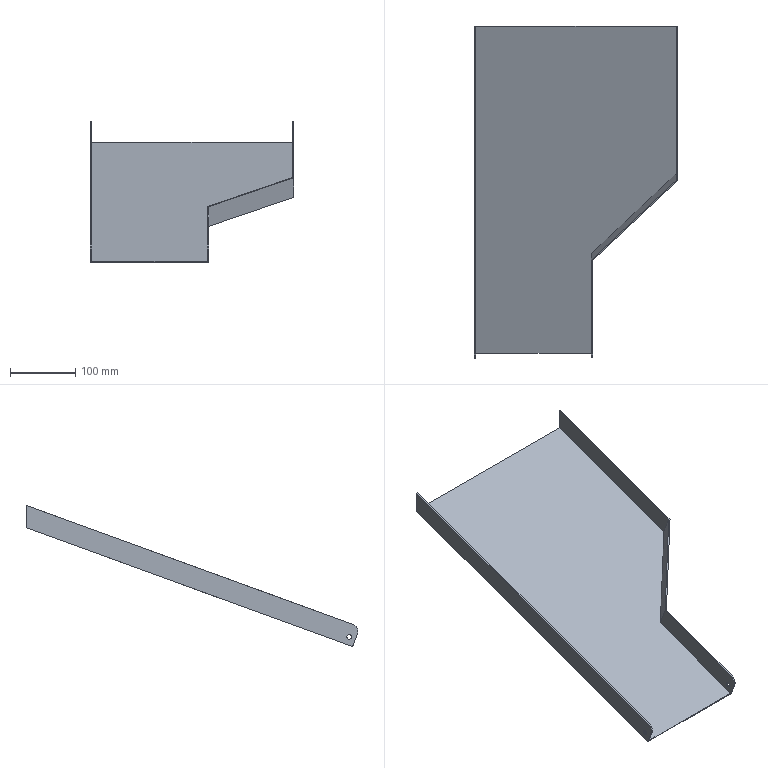Part | NX | features HB 2 | 1 solid | 18 faces | box 311 x 507.033 x 215.64 mm | volume 339071 mm3 | plane 14 | cylinder 4 | commonest cylinder face diameters 7 x2 20 x2
STEP:
#1=CARTESIAN_POINT('',(3094.,-539.252,-364.707));
#2=VERTEX_POINT('',#1);
#3=CARTESIAN_POINT('',(3094.,-691.589,-420.154));
#4=VERTEX_POINT('',#3);
#5=CARTESIAN_POINT('',(3094.,-379.611,-306.603));
#6=DIRECTION('',(0.,-0.9397,-0.342));
#7=VECTOR('',#6,1000.);
#8=LINE('',#5,#7);
#9=EDGE_CURVE('',#2,#4,#8,.T.);
#10=ORIENTED_EDGE('',*,*,#9,.F.);
#11=CARTESIAN_POINT('',(3224.,-417.092,-320.245));
#12=VERTEX_POINT('',#11);
#13=CARTESIAN_POINT('',(3127.943,-507.356,-353.098));
#14=DIRECTION('',(-0.7071,-0.6645,-0.2418));
#15=VECTOR('',#14,1000.);
#16=LINE('',#13,#15);
#17=EDGE_CURVE('',#12,#2,#16,.T.);
#18=ORIENTED_EDGE('',*,*,#17,.F.);
#19=CARTESIAN_POINT('',(3224.,-192.,-238.318));
#20=VERTEX_POINT('',#19);
#21=CARTESIAN_POINT('',(3224.,-379.611,-306.603));
#22=DIRECTION('',(0.,-0.9397,-0.342));
#23=VECTOR('',#22,1000.);
#24=LINE('',#21,#23);
#25=EDGE_CURVE('',#20,#12,#24,.T.);
#26=ORIENTED_EDGE('',*,*,#25,.F.);
#27=CARTESIAN_POINT('',(2917.,-192.,-238.318));
#28=VERTEX_POINT('',#27);
#29=CARTESIAN_POINT('',(2992.,-192.,-238.318));
#30=DIRECTION('',(-1.,0.,0.));
#31=VECTOR('',#30,1000.);
#32=LINE('',#29,#31);
#33=EDGE_CURVE('',#20,#28,#32,.T.);
#34=ORIENTED_EDGE('',*,*,#33,.T.);
#35=CARTESIAN_POINT('',(2917.,-691.589,-420.154));
#36=VERTEX_POINT('',#35);
#37=CARTESIAN_POINT('',(2917.,-379.611,-306.603));
#38=DIRECTION('',(0.,0.9397,0.342));
#39=VECTOR('',#38,1000.);
#40=LINE('',#37,#39);
#41=EDGE_CURVE('',#36,#28,#40,.T.);
#42=ORIENTED_EDGE('',*,*,#41,.F.);
#43=CARTESIAN_POINT('',(2992.,-691.589,-420.154));
#44=DIRECTION('',(1.,0.,0.));
#45=VECTOR('',#44,1000.);
#46=LINE('',#43,#45);
#47=EDGE_CURVE('',#36,#4,#46,.T.);
#48=ORIENTED_EDGE('',*,*,#47,.T.);
#49=EDGE_LOOP('',(#10,#18,#26,#34,#42,#48));
#50=FACE_BOUND('',#49,.T.);
#51=CARTESIAN_POINT('',(2992.,-379.611,-306.603));
#52=DIRECTION('',(0.,-0.342,0.9397));
#53=DIRECTION('',(1.,0.,0.));
#54=AXIS2_PLACEMENT_3D('',#51,#52,#53);
#55=PLANE('',#54);
#56=ADVANCED_FACE('',(#50),#55,.T.);
#57=ORIENTED_EDGE('',*,*,#33,.F.);
#58=CARTESIAN_POINT('',(3224.,-192.,-206.393));
#59=VERTEX_POINT('',#58);
#60=CARTESIAN_POINT('',(3224.,-192.,-306.603));
#61=DIRECTION('',(0.,0.,-1.));
#62=VECTOR('',#61,1000.);
#63=LINE('',#60,#62);
#64=EDGE_CURVE('',#59,#20,#63,.T.);
#65=ORIENTED_EDGE('',*,*,#64,.F.);
#66=CARTESIAN_POINT('',(3226.,-192.,-206.393));
#67=VERTEX_POINT('',#66);
#68=CARTESIAN_POINT('',(3224.,-192.,-206.393));
#69=DIRECTION('',(1.,0.,0.));
#70=VECTOR('',#69,1000.);
#71=LINE('',#68,#70);
#72=EDGE_CURVE('',#59,#67,#71,.T.);
#73=ORIENTED_EDGE('',*,*,#72,.T.);
#74=CARTESIAN_POINT('',(3226.,-192.,-240.446));
#75=VERTEX_POINT('',#74);
#76=CARTESIAN_POINT('',(3226.,-192.,-306.603));
#77=DIRECTION('',(0.,0.,-1.));
#78=VECTOR('',#77,1000.);
#79=LINE('',#76,#78);
#80=EDGE_CURVE('',#67,#75,#79,.T.);
#81=ORIENTED_EDGE('',*,*,#80,.T.);
#82=CARTESIAN_POINT('',(2915.,-192.,-240.446));
#83=VERTEX_POINT('',#82);
#84=CARTESIAN_POINT('',(2992.,-192.,-240.446));
#85=DIRECTION('',(-1.,0.,0.));
#86=VECTOR('',#85,1000.);
#87=LINE('',#84,#86);
#88=EDGE_CURVE('',#75,#83,#87,.T.);
#89=ORIENTED_EDGE('',*,*,#88,.T.);
#90=CARTESIAN_POINT('',(2915.,-192.,-206.393));
#91=VERTEX_POINT('',#90);
#92=CARTESIAN_POINT('',(2915.,-192.,-306.603));
#93=DIRECTION('',(0.,0.,1.));
#94=VECTOR('',#93,1000.);
#95=LINE('',#92,#94);
#96=EDGE_CURVE('',#83,#91,#95,.T.);
#97=ORIENTED_EDGE('',*,*,#96,.T.);
#98=CARTESIAN_POINT('',(2917.,-192.,-206.393));
#99=VERTEX_POINT('',#98);
#100=CARTESIAN_POINT('',(2927.,-192.,-206.393));
#101=DIRECTION('',(1.,0.,0.));
#102=VECTOR('',#101,1000.);
#103=LINE('',#100,#102);
#104=EDGE_CURVE('',#91,#99,#103,.T.);
#105=ORIENTED_EDGE('',*,*,#104,.T.);
#106=CARTESIAN_POINT('',(2917.,-192.,-306.603));
#107=DIRECTION('',(0.,0.,1.));
#108=VECTOR('',#107,1000.);
#109=LINE('',#106,#108);
#110=EDGE_CURVE('',#28,#99,#109,.T.);
#111=ORIENTED_EDGE('',*,*,#110,.F.);
#112=EDGE_LOOP('',(#57,#65,#73,#81,#89,#97,#105,#111));
#113=FACE_BOUND('',#112,.T.);
#114=CARTESIAN_POINT('',(3433.,-192.,70.));
#115=DIRECTION('',(0.,1.,0.));
#116=DIRECTION('',(0.,0.,-1.));
#117=AXIS2_PLACEMENT_3D('',#114,#115,#116);
#118=PLANE('',#117);
#119=ADVANCED_FACE('',(#113),#118,.T.);
#120=CARTESIAN_POINT('',(3226.,-417.186,-322.407));
#121=VERTEX_POINT('',#120);
#122=CARTESIAN_POINT('',(3096.,-539.346,-366.87));
#123=VERTEX_POINT('',#122);
#124=CARTESIAN_POINT('',(3129.357,-508.001,-355.461));
#125=DIRECTION('',(-0.7071,-0.6645,-0.2418));
#126=VECTOR('',#125,1000.);
#127=LINE('',#124,#126);
#128=EDGE_CURVE('',#121,#123,#127,.T.);
#129=ORIENTED_EDGE('',*,*,#128,.T.);
#130=CARTESIAN_POINT('',(3096.,-690.905,-422.033));
#131=VERTEX_POINT('',#130);
#132=CARTESIAN_POINT('',(3096.,-378.927,-308.482));
#133=DIRECTION('',(0.,0.9397,0.342));
#134=VECTOR('',#133,1000.);
#135=LINE('',#132,#134);
#136=EDGE_CURVE('',#131,#123,#135,.T.);
#137=ORIENTED_EDGE('',*,*,#136,.F.);
#138=CARTESIAN_POINT('',(2915.,-690.905,-422.033));
#139=VERTEX_POINT('',#138);
#140=CARTESIAN_POINT('',(2992.,-690.905,-422.033));
#141=DIRECTION('',(1.,0.,0.));
#142=VECTOR('',#141,1000.);
#143=LINE('',#140,#142);
#144=EDGE_CURVE('',#139,#131,#143,.T.);
#145=ORIENTED_EDGE('',*,*,#144,.F.);
#146=CARTESIAN_POINT('',(2915.,-378.927,-308.482));
#147=DIRECTION('',(0.,-0.9397,-0.342));
#148=VECTOR('',#147,1000.);
#149=LINE('',#146,#148);
#150=EDGE_CURVE('',#83,#139,#149,.T.);
#151=ORIENTED_EDGE('',*,*,#150,.F.);
#152=ORIENTED_EDGE('',*,*,#88,.F.);
#153=CARTESIAN_POINT('',(3226.,-378.927,-308.482));
#154=DIRECTION('',(0.,0.9397,0.342));
#155=VECTOR('',#154,1000.);
#156=LINE('',#153,#155);
#157=EDGE_CURVE('',#121,#75,#156,.T.);
#158=ORIENTED_EDGE('',*,*,#157,.F.);
#159=EDGE_LOOP('',(#129,#137,#145,#151,#152,#158));
#160=FACE_BOUND('',#159,.T.);
#161=CARTESIAN_POINT('',(2992.,-378.927,-308.482));
#162=DIRECTION('',(0.,-0.342,0.9397));
#163=DIRECTION('',(1.,0.,0.));
#164=AXIS2_PLACEMENT_3D('',#161,#162,#163);
#165=PLANE('',#164);
#166=ADVANCED_FACE('',(#160),#165,.F.);
#167=CARTESIAN_POINT('',(2915.,-692.453,-388.543));
#168=VERTEX_POINT('',#167);
#169=CARTESIAN_POINT('',(2915.,-389.872,-278.412));
#170=DIRECTION('',(0.,0.9397,0.342));
#171=VECTOR('',#170,1000.);
#172=LINE('',#169,#171);
#173=EDGE_CURVE('',#168,#91,#172,.T.);
#174=ORIENTED_EDGE('',*,*,#173,.F.);
#175=CARTESIAN_POINT('',(2917.,-692.453,-388.543));
#176=VERTEX_POINT('',#175);
#177=CARTESIAN_POINT('',(2927.,-692.453,-388.543));
#178=DIRECTION('',(1.,0.,0.));
#179=VECTOR('',#178,1000.);
#180=LINE('',#177,#179);
#181=EDGE_CURVE('',#168,#176,#180,.T.);
#182=ORIENTED_EDGE('',*,*,#181,.T.);
#183=CARTESIAN_POINT('',(2917.,-389.872,-278.412));
#184=DIRECTION('',(0.,0.9397,0.342));
#185=VECTOR('',#184,1000.);
#186=LINE('',#183,#185);
#187=EDGE_CURVE('',#176,#99,#186,.T.);
#188=ORIENTED_EDGE('',*,*,#187,.T.);
#189=ORIENTED_EDGE('',*,*,#104,.F.);
#190=EDGE_LOOP('',(#174,#182,#188,#189));
#191=FACE_BOUND('',#190,.T.);
#192=CARTESIAN_POINT('',(2927.,-389.872,-278.412));
#193=DIRECTION('',(0.,0.342,-0.9397));
#194=DIRECTION('',(0.,-0.9397,-0.342));
#195=AXIS2_PLACEMENT_3D('',#192,#193,#194);
#196=PLANE('',#195);
#197=ADVANCED_FACE('',(#191),#196,.F.);
#198=ORIENTED_EDGE('',*,*,#187,.F.);
#199=CARTESIAN_POINT('',(2917.,-698.43,-401.36));
#200=VERTEX_POINT('',#199);
#201=CARTESIAN_POINT('',(2917.,-689.033,-397.939));
#202=DIRECTION('',(1.,0.,0.));
#203=DIRECTION('',(0.,0.08716,0.9962));
#204=AXIS2_PLACEMENT_3D('',#201,#202,#203);
#205=CIRCLE('',#204,10.);
#206=EDGE_CURVE('',#176,#200,#205,.T.);
#207=ORIENTED_EDGE('',*,*,#206,.T.);
#208=CARTESIAN_POINT('',(2917.,-691.589,-420.154));
#209=DIRECTION('',(0.,-0.342,0.9397));
#210=VECTOR('',#209,1000.);
#211=LINE('',#208,#210);
#212=EDGE_CURVE('',#36,#200,#211,.T.);
#213=ORIENTED_EDGE('',*,*,#212,.F.);
#214=ORIENTED_EDGE('',*,*,#41,.T.);
#215=ORIENTED_EDGE('',*,*,#110,.T.);
#216=EDGE_LOOP('',(#198,#207,#213,#214,#215));
#217=FACE_BOUND('',#216,.T.);
#218=CARTESIAN_POINT('',(2917.,-685.307,-403.85));
#219=VERTEX_POINT('',#218);
#220=CARTESIAN_POINT('',(2917.,-685.612,-407.336));
#221=DIRECTION('',(-1.,0.,0.));
#222=DIRECTION('',(0.,0.08716,0.9962));
#223=AXIS2_PLACEMENT_3D('',#220,#221,#222);
#224=CIRCLE('',#223,3.5);
#225=EDGE_CURVE('',#219,#219,#224,.T.);
#226=ORIENTED_EDGE('',*,*,#225,.T.);
#227=EDGE_LOOP('',(#226));
#228=FACE_BOUND('',#227,.T.);
#229=CARTESIAN_POINT('',(2917.,-379.611,-306.603));
#230=DIRECTION('',(1.,0.,0.));
#231=DIRECTION('',(0.,0.08716,0.9962));
#232=AXIS2_PLACEMENT_3D('',#229,#230,#231);
#233=PLANE('',#232);
#234=ADVANCED_FACE('',(#217,#228),#233,.T.);
#235=CARTESIAN_POINT('',(3096.,-550.291,-336.8));
#236=VERTEX_POINT('',#235);
#237=CARTESIAN_POINT('',(3226.,-428.131,-292.337));
#238=VERTEX_POINT('',#237);
#239=CARTESIAN_POINT('',(3245.357,-409.941,-285.717));
#240=DIRECTION('',(0.7071,0.6645,0.2418));
#241=VECTOR('',#240,1000.);
#242=LINE('',#239,#241);
#243=EDGE_CURVE('',#236,#238,#242,.T.);
#244=ORIENTED_EDGE('',*,*,#243,.T.);
#245=CARTESIAN_POINT('',(3226.,-389.872,-278.412));
#246=DIRECTION('',(0.,0.9397,0.342));
#247=VECTOR('',#246,1000.);
#248=LINE('',#245,#247);
#249=EDGE_CURVE('',#238,#67,#248,.T.);
#250=ORIENTED_EDGE('',*,*,#249,.T.);
#251=ORIENTED_EDGE('',*,*,#72,.F.);
#252=CARTESIAN_POINT('',(3224.,-427.353,-292.054));
#253=VERTEX_POINT('',#252);
#254=CARTESIAN_POINT('',(3224.,-389.872,-278.412));
#255=DIRECTION('',(0.,0.9397,0.342));
#256=VECTOR('',#255,1000.);
#257=LINE('',#254,#256);
#258=EDGE_CURVE('',#253,#59,#257,.T.);
#259=ORIENTED_EDGE('',*,*,#258,.F.);
#260=CARTESIAN_POINT('',(3094.,-549.513,-336.517));
#261=VERTEX_POINT('',#260);
#262=CARTESIAN_POINT('',(3243.943,-408.612,-285.233));
#263=DIRECTION('',(0.7071,0.6645,0.2418));
#264=VECTOR('',#263,1000.);
#265=LINE('',#262,#264);
#266=EDGE_CURVE('',#261,#253,#265,.T.);
#267=ORIENTED_EDGE('',*,*,#266,.F.);
#268=CARTESIAN_POINT('',(3094.,-692.453,-388.543));
#269=VERTEX_POINT('',#268);
#270=CARTESIAN_POINT('',(3094.,-389.872,-278.412));
#271=DIRECTION('',(0.,0.9397,0.342));
#272=VECTOR('',#271,1000.);
#273=LINE('',#270,#272);
#274=EDGE_CURVE('',#269,#261,#273,.T.);
#275=ORIENTED_EDGE('',*,*,#274,.F.);
#276=CARTESIAN_POINT('',(3096.,-692.453,-388.543));
#277=VERTEX_POINT('',#276);
#278=CARTESIAN_POINT('',(3224.,-692.453,-388.543));
#279=DIRECTION('',(1.,0.,0.));
#280=VECTOR('',#279,1000.);
#281=LINE('',#278,#280);
#282=EDGE_CURVE('',#269,#277,#281,.T.);
#283=ORIENTED_EDGE('',*,*,#282,.T.);
#284=CARTESIAN_POINT('',(3096.,-389.872,-278.412));
#285=DIRECTION('',(0.,0.9397,0.342));
#286=VECTOR('',#285,1000.);
#287=LINE('',#284,#286);
#288=EDGE_CURVE('',#277,#236,#287,.T.);
#289=ORIENTED_EDGE('',*,*,#288,.T.);
#290=EDGE_LOOP('',(#244,#250,#251,#259,#267,#275,#283,#289));
#291=FACE_BOUND('',#290,.T.);
#292=CARTESIAN_POINT('',(3224.,-389.872,-278.412));
#293=DIRECTION('',(0.,0.342,-0.9397));
#294=DIRECTION('',(0.,-0.9397,-0.342));
#295=AXIS2_PLACEMENT_3D('',#292,#293,#294);
#296=PLANE('',#295);
#297=ADVANCED_FACE('',(#291),#296,.F.);
#298=CARTESIAN_POINT('',(3224.,-417.092,-320.245));
#299=DIRECTION('',(0.,0.342,-0.9397));
#300=VECTOR('',#299,1000.);
#301=LINE('',#298,#300);
#302=EDGE_CURVE('',#253,#12,#301,.T.);
#303=ORIENTED_EDGE('',*,*,#302,.F.);
#304=ORIENTED_EDGE('',*,*,#258,.T.);
#305=ORIENTED_EDGE('',*,*,#64,.T.);
#306=ORIENTED_EDGE('',*,*,#25,.T.);
#307=EDGE_LOOP('',(#303,#304,#305,#306));
#308=FACE_BOUND('',#307,.T.);
#309=CARTESIAN_POINT('',(3224.,-379.611,-306.603));
#310=DIRECTION('',(-1.,0.,0.));
#311=DIRECTION('',(0.,0.08716,0.9962));
#312=AXIS2_PLACEMENT_3D('',#309,#310,#311);
#313=PLANE('',#312);
#314=ADVANCED_FACE('',(#308),#313,.T.);
#315=ORIENTED_EDGE('',*,*,#249,.F.);
#316=CARTESIAN_POINT('',(3226.,-417.87,-320.528));
#317=DIRECTION('',(0.,-0.342,0.9397));
#318=VECTOR('',#317,1000.);
#319=LINE('',#316,#318);
#320=EDGE_CURVE('',#121,#238,#319,.T.);
#321=ORIENTED_EDGE('',*,*,#320,.F.);
#322=ORIENTED_EDGE('',*,*,#157,.T.);
#323=ORIENTED_EDGE('',*,*,#80,.F.);
#324=EDGE_LOOP('',(#315,#321,#322,#323));
#325=FACE_BOUND('',#324,.T.);
#326=CARTESIAN_POINT('',(3226.,-379.611,-306.603));
#327=DIRECTION('',(-1.,0.,0.));
#328=DIRECTION('',(0.,0.08716,0.9962));
#329=AXIS2_PLACEMENT_3D('',#326,#327,#328);
#330=PLANE('',#329);
#331=ADVANCED_FACE('',(#325),#330,.F.);
#332=ORIENTED_EDGE('',*,*,#150,.T.);
#333=CARTESIAN_POINT('',(2915.,-698.43,-401.36));
#334=VERTEX_POINT('',#333);
#335=CARTESIAN_POINT('',(2915.,-691.589,-420.154));
#336=DIRECTION('',(0.,-0.342,0.9397));
#337=VECTOR('',#336,1000.);
#338=LINE('',#335,#337);
#339=EDGE_CURVE('',#139,#334,#338,.T.);
#340=ORIENTED_EDGE('',*,*,#339,.T.);
#341=CARTESIAN_POINT('',(2915.,-689.033,-397.939));
#342=DIRECTION('',(-1.,0.,0.));
#343=DIRECTION('',(0.,0.08716,0.9962));
#344=AXIS2_PLACEMENT_3D('',#341,#342,#343);
#345=CIRCLE('',#344,10.);
#346=EDGE_CURVE('',#334,#168,#345,.T.);
#347=ORIENTED_EDGE('',*,*,#346,.T.);
#348=ORIENTED_EDGE('',*,*,#173,.T.);
#349=ORIENTED_EDGE('',*,*,#96,.F.);
#350=EDGE_LOOP('',(#332,#340,#347,#348,#349));
#351=FACE_BOUND('',#350,.T.);
#352=CARTESIAN_POINT('',(2915.,-685.307,-403.85));
#353=VERTEX_POINT('',#352);
#354=CARTESIAN_POINT('',(2915.,-685.612,-407.336));
#355=DIRECTION('',(-1.,0.,0.));
#356=DIRECTION('',(0.,0.08716,0.9962));
#357=AXIS2_PLACEMENT_3D('',#354,#355,#356);
#358=CIRCLE('',#357,3.5);
#359=EDGE_CURVE('',#353,#353,#358,.T.);
#360=ORIENTED_EDGE('',*,*,#359,.F.);
#361=EDGE_LOOP('',(#360));
#362=FACE_BOUND('',#361,.T.);
#363=CARTESIAN_POINT('',(2915.,-379.611,-306.603));
#364=DIRECTION('',(1.,0.,0.));
#365=DIRECTION('',(0.,-0.08716,-0.9962));
#366=AXIS2_PLACEMENT_3D('',#363,#364,#365);
#367=PLANE('',#366);
#368=ADVANCED_FACE('',(#351,#362),#367,.F.);
#369=CARTESIAN_POINT('',(3096.,-685.918,-410.823));
#370=VERTEX_POINT('',#369);
#371=CARTESIAN_POINT('',(3096.,-685.612,-407.336));
#372=DIRECTION('',(-1.,0.,0.));
#373=DIRECTION('',(0.,-0.08716,-0.9962));
#374=AXIS2_PLACEMENT_3D('',#371,#372,#373);
#375=CIRCLE('',#374,3.5);
#376=EDGE_CURVE('',#370,#370,#375,.T.);
#377=ORIENTED_EDGE('',*,*,#376,.T.);
#378=EDGE_LOOP('',(#377));
#379=FACE_BOUND('',#378,.T.);
#380=ORIENTED_EDGE('',*,*,#136,.T.);
#381=CARTESIAN_POINT('',(3096.,-540.03,-364.991));
#382=DIRECTION('',(0.,-0.342,0.9397));
#383=VECTOR('',#382,1000.);
#384=LINE('',#381,#383);
#385=EDGE_CURVE('',#123,#236,#384,.T.);
#386=ORIENTED_EDGE('',*,*,#385,.T.);
#387=ORIENTED_EDGE('',*,*,#288,.F.);
#388=CARTESIAN_POINT('',(3096.,-698.43,-401.36));
#389=VERTEX_POINT('',#388);
#390=CARTESIAN_POINT('',(3096.,-689.033,-397.939));
#391=DIRECTION('',(1.,0.,0.));
#392=DIRECTION('',(0.,-0.08716,-0.9962));
#393=AXIS2_PLACEMENT_3D('',#390,#391,#392);
#394=CIRCLE('',#393,10.);
#395=EDGE_CURVE('',#277,#389,#394,.T.);
#396=ORIENTED_EDGE('',*,*,#395,.T.);
#397=CARTESIAN_POINT('',(3096.,-691.589,-420.154));
#398=DIRECTION('',(0.,-0.342,0.9397));
#399=VECTOR('',#398,1000.);
#400=LINE('',#397,#399);
#401=EDGE_CURVE('',#131,#389,#400,.T.);
#402=ORIENTED_EDGE('',*,*,#401,.F.);
#403=EDGE_LOOP('',(#380,#386,#387,#396,#402));
#404=FACE_BOUND('',#403,.T.);
#405=CARTESIAN_POINT('',(3096.,-379.611,-306.603));
#406=DIRECTION('',(-1.,0.,0.));
#407=DIRECTION('',(0.,0.08716,0.9962));
#408=AXIS2_PLACEMENT_3D('',#405,#406,#407);
#409=PLANE('',#408);
#410=ADVANCED_FACE('',(#379,#404),#409,.F.);
#411=CARTESIAN_POINT('',(3094.,-685.918,-410.823));
#412=VERTEX_POINT('',#411);
#413=CARTESIAN_POINT('',(3094.,-685.612,-407.336));
#414=DIRECTION('',(1.,0.,0.));
#415=DIRECTION('',(0.,-0.08716,-0.9962));
#416=AXIS2_PLACEMENT_3D('',#413,#414,#415);
#417=CIRCLE('',#416,3.5);
#418=EDGE_CURVE('',#412,#412,#417,.T.);
#419=ORIENTED_EDGE('',*,*,#418,.T.);
#420=EDGE_LOOP('',(#419));
#421=FACE_BOUND('',#420,.T.);
#422=ORIENTED_EDGE('',*,*,#274,.T.);
#423=CARTESIAN_POINT('',(3094.,-539.252,-364.707));
#424=DIRECTION('',(0.,-0.342,0.9397));
#425=VECTOR('',#424,1000.);
#426=LINE('',#423,#425);
#427=EDGE_CURVE('',#2,#261,#426,.T.);
#428=ORIENTED_EDGE('',*,*,#427,.F.);
#429=ORIENTED_EDGE('',*,*,#9,.T.);
#430=CARTESIAN_POINT('',(3094.,-698.43,-401.36));
#431=VERTEX_POINT('',#430);
#432=CARTESIAN_POINT('',(3094.,-691.589,-420.154));
#433=DIRECTION('',(0.,-0.342,0.9397));
#434=VECTOR('',#433,1000.);
#435=LINE('',#432,#434);
#436=EDGE_CURVE('',#4,#431,#435,.T.);
#437=ORIENTED_EDGE('',*,*,#436,.T.);
#438=CARTESIAN_POINT('',(3094.,-689.033,-397.939));
#439=DIRECTION('',(-1.,0.,0.));
#440=DIRECTION('',(0.,-0.08716,-0.9962));
#441=AXIS2_PLACEMENT_3D('',#438,#439,#440);
#442=CIRCLE('',#441,10.);
#443=EDGE_CURVE('',#431,#269,#442,.T.);
#444=ORIENTED_EDGE('',*,*,#443,.T.);
#445=EDGE_LOOP('',(#422,#428,#429,#437,#444));
#446=FACE_BOUND('',#445,.T.);
#447=CARTESIAN_POINT('',(3094.,-379.611,-306.603));
#448=DIRECTION('',(-1.,0.,0.));
#449=DIRECTION('',(0.,0.08716,0.9962));
#450=AXIS2_PLACEMENT_3D('',#447,#448,#449);
#451=PLANE('',#450);
#452=ADVANCED_FACE('',(#421,#446),#451,.T.);
#453=ORIENTED_EDGE('',*,*,#339,.F.);
#454=ORIENTED_EDGE('',*,*,#144,.T.);
#455=ORIENTED_EDGE('',*,*,#401,.T.);
#456=CARTESIAN_POINT('',(2966.,-698.43,-401.36));
#457=DIRECTION('',(-1.,0.,0.));
#458=VECTOR('',#457,1000.);
#459=LINE('',#456,#458);
#460=EDGE_CURVE('',#389,#431,#459,.T.);
#461=ORIENTED_EDGE('',*,*,#460,.T.);
#462=ORIENTED_EDGE('',*,*,#436,.F.);
#463=ORIENTED_EDGE('',*,*,#47,.F.);
#464=ORIENTED_EDGE('',*,*,#212,.T.);
#465=CARTESIAN_POINT('',(2992.,-698.43,-401.36));
#466=DIRECTION('',(-1.,0.,0.));
#467=VECTOR('',#466,1000.);
#468=LINE('',#465,#467);
#469=EDGE_CURVE('',#200,#334,#468,.T.);
#470=ORIENTED_EDGE('',*,*,#469,.T.);
#471=EDGE_LOOP('',(#453,#454,#455,#461,#462,#463,#464,#470));
#472=FACE_BOUND('',#471,.T.);
#473=CARTESIAN_POINT('',(2992.,-691.589,-420.154));
#474=DIRECTION('',(0.,0.9397,0.342));
#475=DIRECTION('',(0.,0.342,-0.9397));
#476=AXIS2_PLACEMENT_3D('',#473,#474,#475);
#477=PLANE('',#476);
#478=ADVANCED_FACE('',(#472),#477,.F.);
#479=ORIENTED_EDGE('',*,*,#206,.F.);
#480=ORIENTED_EDGE('',*,*,#181,.F.);
#481=ORIENTED_EDGE('',*,*,#346,.F.);
#482=ORIENTED_EDGE('',*,*,#469,.F.);
#483=EDGE_LOOP('',(#479,#480,#481,#482));
#484=FACE_BOUND('',#483,.T.);
#485=CARTESIAN_POINT('',(2927.,-689.033,-397.939));
#486=DIRECTION('',(-1.,0.,0.));
#487=DIRECTION('',(0.,0.08716,0.9962));
#488=AXIS2_PLACEMENT_3D('',#485,#486,#487);
#489=CYLINDRICAL_SURFACE('',#488,10.);
#490=ADVANCED_FACE('',(#484),#489,.T.);
#491=ORIENTED_EDGE('',*,*,#443,.F.);
#492=ORIENTED_EDGE('',*,*,#460,.F.);
#493=ORIENTED_EDGE('',*,*,#395,.F.);
#494=ORIENTED_EDGE('',*,*,#282,.F.);
#495=EDGE_LOOP('',(#491,#492,#493,#494));
#496=FACE_BOUND('',#495,.T.);
#497=CARTESIAN_POINT('',(2966.,-689.033,-397.939));
#498=DIRECTION('',(1.,0.,0.));
#499=DIRECTION('',(0.,-0.08716,-0.9962));
#500=AXIS2_PLACEMENT_3D('',#497,#498,#499);
#501=CYLINDRICAL_SURFACE('',#500,10.);
#502=ADVANCED_FACE('',(#496),#501,.T.);
#503=ORIENTED_EDGE('',*,*,#225,.F.);
#504=EDGE_LOOP('',(#503));
#505=FACE_BOUND('',#504,.T.);
#506=ORIENTED_EDGE('',*,*,#359,.T.);
#507=EDGE_LOOP('',(#506));
#508=FACE_BOUND('',#507,.T.);
#509=CARTESIAN_POINT('',(2323.,-685.612,-407.336));
#510=DIRECTION('',(1.,0.,0.));
#511=DIRECTION('',(0.,-0.08716,-0.9962));
#512=AXIS2_PLACEMENT_3D('',#509,#510,#511);
#513=CYLINDRICAL_SURFACE('',#512,3.5);
#514=ADVANCED_FACE('',(#505,#508),#513,.F.);
#515=ORIENTED_EDGE('',*,*,#418,.F.);
#516=EDGE_LOOP('',(#515));
#517=FACE_BOUND('',#516,.T.);
#518=ORIENTED_EDGE('',*,*,#376,.F.);
#519=EDGE_LOOP('',(#518));
#520=FACE_BOUND('',#519,.T.);
#521=CARTESIAN_POINT('',(2374.,-685.612,-407.336));
#522=DIRECTION('',(1.,0.,0.));
#523=DIRECTION('',(0.,-0.08716,-0.9962));
#524=AXIS2_PLACEMENT_3D('',#521,#522,#523);
#525=CYLINDRICAL_SURFACE('',#524,3.5);
#526=ADVANCED_FACE('',(#517,#520),#525,.F.);
#527=ORIENTED_EDGE('',*,*,#385,.F.);
#528=ORIENTED_EDGE('',*,*,#128,.F.);
#529=ORIENTED_EDGE('',*,*,#320,.T.);
#530=ORIENTED_EDGE('',*,*,#243,.F.);
#531=EDGE_LOOP('',(#527,#528,#529,#530));
#532=FACE_BOUND('',#531,.T.);
#533=CARTESIAN_POINT('',(3226.,-428.131,-292.337));
#534=DIRECTION('',(0.7071,-0.6645,-0.2418));
#535=DIRECTION('',(0.,0.342,-0.9397));
#536=AXIS2_PLACEMENT_3D('',#533,#534,#535);
#537=PLANE('',#536);
#538=ADVANCED_FACE('',(#532),#537,.T.);
#539=ORIENTED_EDGE('',*,*,#302,.T.);
#540=ORIENTED_EDGE('',*,*,#17,.T.);
#541=ORIENTED_EDGE('',*,*,#427,.T.);
#542=ORIENTED_EDGE('',*,*,#266,.T.);
#543=EDGE_LOOP('',(#539,#540,#541,#542));
#544=FACE_BOUND('',#543,.T.);
#545=CARTESIAN_POINT('',(3224.586,-426.802,-291.854));
#546=DIRECTION('',(0.7071,-0.6645,-0.2418));
#547=DIRECTION('',(0.,0.342,-0.9397));
#548=AXIS2_PLACEMENT_3D('',#545,#546,#547);
#549=PLANE('',#548);
#550=ADVANCED_FACE('',(#544),#549,.F.);
#551=CLOSED_SHELL('',(#56,#119,#166,#197,#234,#297,#314,#331,#368,#410,#452,#478,#490,#502,#514,#526,#538,#550));
#552=MANIFOLD_SOLID_BREP('',#551);
#553=(LENGTH_UNIT()NAMED_UNIT(*)SI_UNIT(.MILLI.,.METRE.));
#554=UNCERTAINTY_MEASURE_WITH_UNIT(LENGTH_MEASURE(0.00001),#553,'','');
#555=(NAMED_UNIT(*)PLANE_ANGLE_UNIT()SI_UNIT($,.RADIAN.));
#556=(NAMED_UNIT(*)SI_UNIT($,.STERADIAN.)SOLID_ANGLE_UNIT());
#557=(GEOMETRIC_REPRESENTATION_CONTEXT(3)GLOBAL_UNCERTAINTY_ASSIGNED_CONTEXT((#554))GLOBAL_UNIT_ASSIGNED_CONTEXT((#553,#555,#556))REPRESENTATION_CONTEXT('',''));
#558=ADVANCED_BREP_SHAPE_REPRESENTATION('',(#552),#557);